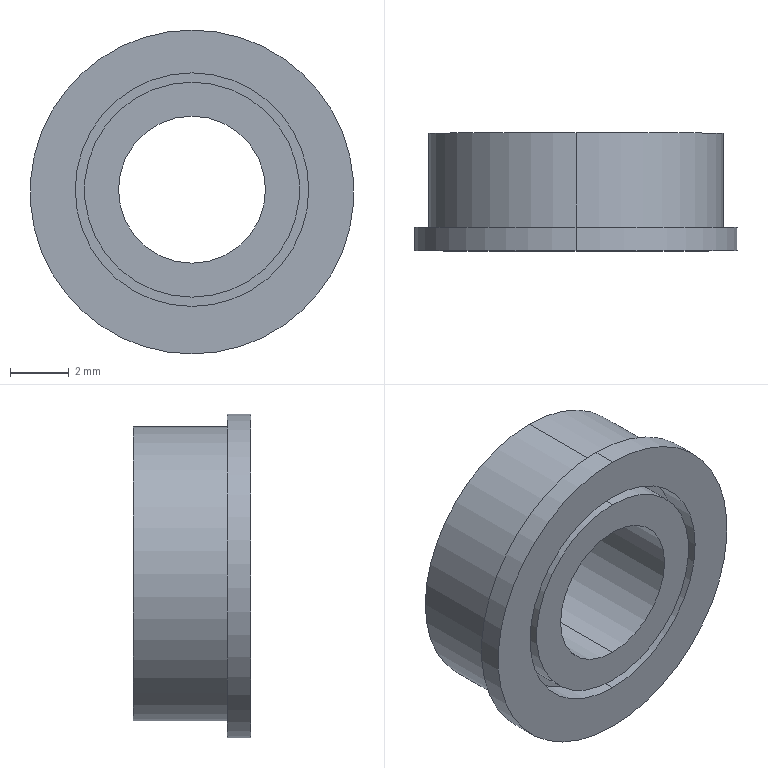Part | STEP file | Flange bearing 5104 | 1 solid | 21 faces | box 11 x 4 x 11 mm | volume 233.729 mm3 | cylinder 14 | plane 7 | commonest cylinder face diameters 7.305 x4 7.935 x4 5 x2 10 x2 11 x2
STEP:
#1=CARTESIAN_POINT('',(0.,0.,0.));
#2=DIRECTION('',(0.,0.,1.));
#3=DIRECTION('',(1.,0.,0.));
#4=AXIS2_PLACEMENT_3D('',#1,#2,#3);
#5=CARTESIAN_POINT('',(0.,1.,-3.653));
#6=VERTEX_POINT('',#5);
#7=CARTESIAN_POINT('',(0.,1.,3.653));
#8=VERTEX_POINT('',#7);
#9=CARTESIAN_POINT('',(0.,1.,0.));
#10=DIRECTION('',(0.,-1.,0.));
#11=DIRECTION('',(0.,0.,-1.));
#12=AXIS2_PLACEMENT_3D('',#9,#10,#11);
#13=CIRCLE('',#12,3.653);
#14=CARTESIAN_POINT('',(0.,1.,0.));
#15=DIRECTION('',(0.,-1.,0.));
#16=DIRECTION('',(0.,0.,-1.));
#17=AXIS2_PLACEMENT_3D('',#14,#15,#16);
#18=CYLINDRICAL_SURFACE('',#17,3.653);
#19=CARTESIAN_POINT('',(0.,0.));
#20=DIRECTION('',(1.,0.));
#21=VECTOR('',#20,1.);
#22=LINE('',#19,#21);
#23=(GEOMETRIC_REPRESENTATION_CONTEXT(2)PARAMETRIC_REPRESENTATION_CONTEXT()REPRESENTATION_CONTEXT('',''));
#24=DEFINITIONAL_REPRESENTATION('',(#22),#23);
#25=PCURVE('',#18,#24);
#26=CARTESIAN_POINT('',(0.,1.,0.));
#27=DIRECTION('',(0.,-1.,0.));
#28=DIRECTION('',(0.,0.,-1.));
#29=AXIS2_PLACEMENT_3D('',#26,#27,#28);
#30=PLANE('',#29);
#31=CARTESIAN_POINT('',(0.,0.));
#32=DIRECTION('',(1.,0.));
#33=AXIS2_PLACEMENT_2D('',#31,#32);
#34=CIRCLE('',#33,3.653);
#35=(GEOMETRIC_REPRESENTATION_CONTEXT(2)PARAMETRIC_REPRESENTATION_CONTEXT()REPRESENTATION_CONTEXT('',''));
#36=DEFINITIONAL_REPRESENTATION('',(#34),#35);
#37=PCURVE('',#30,#36);
#38=SURFACE_CURVE('',#13,(#25,#37),.PCURVE_S1.);
#39=EDGE_CURVE('',#6,#8,#38,.T.);
#40=ORIENTED_EDGE('',*,*,#39,.T.);
#41=CARTESIAN_POINT('',(0.,0.,3.653));
#42=VERTEX_POINT('',#41);
#43=CARTESIAN_POINT('',(0.,1.,3.653));
#44=DIRECTION('',(0.,-1.,0.));
#45=VECTOR('',#44,1.);
#46=LINE('',#43,#45);
#47=CARTESIAN_POINT('',(3.142,0.));
#48=DIRECTION('',(0.,1.));
#49=VECTOR('',#48,1.);
#50=LINE('',#47,#49);
#51=(GEOMETRIC_REPRESENTATION_CONTEXT(2)PARAMETRIC_REPRESENTATION_CONTEXT()REPRESENTATION_CONTEXT('',''));
#52=DEFINITIONAL_REPRESENTATION('',(#50),#51);
#53=PCURVE('',#18,#52);
#54=CARTESIAN_POINT('',(0.,1.,0.));
#55=DIRECTION('',(0.,-1.,0.));
#56=DIRECTION('',(0.,0.,-1.));
#57=AXIS2_PLACEMENT_3D('',#54,#55,#56);
#58=CYLINDRICAL_SURFACE('',#57,3.653);
#59=CARTESIAN_POINT('',(3.142,0.));
#60=DIRECTION('',(0.,1.));
#61=VECTOR('',#60,1.);
#62=LINE('',#59,#61);
#63=(GEOMETRIC_REPRESENTATION_CONTEXT(2)PARAMETRIC_REPRESENTATION_CONTEXT()REPRESENTATION_CONTEXT('',''));
#64=DEFINITIONAL_REPRESENTATION('',(#62),#63);
#65=PCURVE('',#58,#64);
#66=SURFACE_CURVE('',#46,(#53,#65),.PCURVE_S1.);
#67=EDGE_CURVE('',#8,#42,#66,.T.);
#68=ORIENTED_EDGE('',*,*,#67,.T.);
#69=CARTESIAN_POINT('',(0.,0.,-3.653));
#70=VERTEX_POINT('',#69);
#71=CARTESIAN_POINT('',(0.,0.,0.));
#72=DIRECTION('',(0.,-1.,0.));
#73=DIRECTION('',(0.,0.,-1.));
#74=AXIS2_PLACEMENT_3D('',#71,#72,#73);
#75=CIRCLE('',#74,3.653);
#76=CARTESIAN_POINT('',(0.,1.));
#77=DIRECTION('',(1.,0.));
#78=VECTOR('',#77,1.);
#79=LINE('',#76,#78);
#80=(GEOMETRIC_REPRESENTATION_CONTEXT(2)PARAMETRIC_REPRESENTATION_CONTEXT()REPRESENTATION_CONTEXT('',''));
#81=DEFINITIONAL_REPRESENTATION('',(#79),#80);
#82=PCURVE('',#18,#81);
#83=CARTESIAN_POINT('',(0.,0.,0.));
#84=DIRECTION('',(0.,1.,0.));
#85=DIRECTION('',(0.,0.,1.));
#86=AXIS2_PLACEMENT_3D('',#83,#84,#85);
#87=PLANE('',#86);
#88=CARTESIAN_POINT('',(-3.653,0.));
#89=CARTESIAN_POINT('',(-3.653,6.326));
#90=CARTESIAN_POINT('',(1.826,3.163));
#91=CARTESIAN_POINT('',(7.305,0.));
#92=CARTESIAN_POINT('',(1.826,-3.163));
#93=CARTESIAN_POINT('',(-3.653,-6.326));
#94=CARTESIAN_POINT('',(-3.653,0.));
#95=(BOUNDED_CURVE()B_SPLINE_CURVE(2,(#88,#89,#90,#91,#92,#93,#94),.UNSPECIFIED.,.T.,.F.)B_SPLINE_CURVE_WITH_KNOTS((1,2,2,2,2,1),(-2.094,0.,2.094,4.189,6.283,8.378),.UNSPECIFIED.)CURVE()GEOMETRIC_REPRESENTATION_ITEM()RATIONAL_B_SPLINE_CURVE((1.,0.5,1.,0.5,1.,0.5,1.))REPRESENTATION_ITEM(''));
#96=(GEOMETRIC_REPRESENTATION_CONTEXT(2)PARAMETRIC_REPRESENTATION_CONTEXT()REPRESENTATION_CONTEXT('',''));
#97=DEFINITIONAL_REPRESENTATION('',(#95),#96);
#98=PCURVE('',#87,#97);
#99=SURFACE_CURVE('',#75,(#82,#98),.PCURVE_S1.);
#100=EDGE_CURVE('',#70,#42,#99,.T.);
#101=ORIENTED_EDGE('',*,*,#100,.F.);
#102=CARTESIAN_POINT('',(0.,1.,-3.653));
#103=DIRECTION('',(0.,-1.,0.));
#104=VECTOR('',#103,1.);
#105=LINE('',#102,#104);
#106=CARTESIAN_POINT('',(0.,0.));
#107=DIRECTION('',(0.,1.));
#108=VECTOR('',#107,1.);
#109=LINE('',#106,#108);
#110=(GEOMETRIC_REPRESENTATION_CONTEXT(2)PARAMETRIC_REPRESENTATION_CONTEXT()REPRESENTATION_CONTEXT('',''));
#111=DEFINITIONAL_REPRESENTATION('',(#109),#110);
#112=PCURVE('',#18,#111);
#113=CARTESIAN_POINT('',(6.283,0.));
#114=DIRECTION('',(0.,1.));
#115=VECTOR('',#114,1.);
#116=LINE('',#113,#115);
#117=(GEOMETRIC_REPRESENTATION_CONTEXT(2)PARAMETRIC_REPRESENTATION_CONTEXT()REPRESENTATION_CONTEXT('',''));
#118=DEFINITIONAL_REPRESENTATION('',(#116),#117);
#119=PCURVE('',#58,#118);
#120=SURFACE_CURVE('',#105,(#112,#119),.PCURVE_S1.);
#121=EDGE_CURVE('',#6,#70,#120,.T.);
#122=ORIENTED_EDGE('',*,*,#121,.F.);
#123=EDGE_LOOP('',(#40,#68,#101,#122));
#124=FACE_BOUND('',#123,.T.);
#125=ADVANCED_FACE('',(#124),#18,.T.);
#126=CARTESIAN_POINT('',(0.,1.,-3.968));
#127=VERTEX_POINT('',#126);
#128=CARTESIAN_POINT('',(0.,0.,-3.968));
#129=VERTEX_POINT('',#128);
#130=CARTESIAN_POINT('',(0.,1.,-3.968));
#131=DIRECTION('',(0.,-1.,0.));
#132=VECTOR('',#131,1.);
#133=LINE('',#130,#132);
#134=CARTESIAN_POINT('',(0.,1.,0.));
#135=DIRECTION('',(0.,-1.,0.));
#136=DIRECTION('',(0.,0.,-1.));
#137=AXIS2_PLACEMENT_3D('',#134,#135,#136);
#138=CYLINDRICAL_SURFACE('',#137,3.968);
#139=CARTESIAN_POINT('',(6.283,0.));
#140=DIRECTION('',(0.,1.));
#141=VECTOR('',#140,1.);
#142=LINE('',#139,#141);
#143=(GEOMETRIC_REPRESENTATION_CONTEXT(2)PARAMETRIC_REPRESENTATION_CONTEXT()REPRESENTATION_CONTEXT('',''));
#144=DEFINITIONAL_REPRESENTATION('',(#142),#143);
#145=PCURVE('',#138,#144);
#146=CARTESIAN_POINT('',(0.,1.,0.));
#147=DIRECTION('',(0.,-1.,0.));
#148=DIRECTION('',(0.,0.,-1.));
#149=AXIS2_PLACEMENT_3D('',#146,#147,#148);
#150=CYLINDRICAL_SURFACE('',#149,3.968);
#151=CARTESIAN_POINT('',(0.,0.));
#152=DIRECTION('',(0.,1.));
#153=VECTOR('',#152,1.);
#154=LINE('',#151,#153);
#155=(GEOMETRIC_REPRESENTATION_CONTEXT(2)PARAMETRIC_REPRESENTATION_CONTEXT()REPRESENTATION_CONTEXT('',''));
#156=DEFINITIONAL_REPRESENTATION('',(#154),#155);
#157=PCURVE('',#150,#156);
#158=SURFACE_CURVE('',#133,(#145,#157),.PCURVE_S1.);
#159=EDGE_CURVE('',#127,#129,#158,.T.);
#160=ORIENTED_EDGE('',*,*,#159,.T.);
#161=CARTESIAN_POINT('',(0.,0.,3.968));
#162=VERTEX_POINT('',#161);
#163=CARTESIAN_POINT('',(0.,0.,0.));
#164=DIRECTION('',(0.,-1.,0.));
#165=DIRECTION('',(0.,0.,-1.));
#166=AXIS2_PLACEMENT_3D('',#163,#164,#165);
#167=CIRCLE('',#166,3.968);
#168=CARTESIAN_POINT('',(0.,1.));
#169=DIRECTION('',(1.,0.));
#170=VECTOR('',#169,1.);
#171=LINE('',#168,#170);
#172=(GEOMETRIC_REPRESENTATION_CONTEXT(2)PARAMETRIC_REPRESENTATION_CONTEXT()REPRESENTATION_CONTEXT('',''));
#173=DEFINITIONAL_REPRESENTATION('',(#171),#172);
#174=PCURVE('',#138,#173);
#175=CARTESIAN_POINT('',(0.,0.,0.));
#176=DIRECTION('',(0.,1.,0.));
#177=DIRECTION('',(0.,0.,1.));
#178=AXIS2_PLACEMENT_3D('',#175,#176,#177);
#179=PLANE('',#178);
#180=CARTESIAN_POINT('',(-3.968,0.));
#181=CARTESIAN_POINT('',(-3.968,6.872));
#182=CARTESIAN_POINT('',(1.984,3.436));
#183=CARTESIAN_POINT('',(7.935,0.));
#184=CARTESIAN_POINT('',(1.984,-3.436));
#185=CARTESIAN_POINT('',(-3.968,-6.872));
#186=CARTESIAN_POINT('',(-3.968,0.));
#187=(BOUNDED_CURVE()B_SPLINE_CURVE(2,(#180,#181,#182,#183,#184,#185,#186),.UNSPECIFIED.,.T.,.F.)B_SPLINE_CURVE_WITH_KNOTS((1,2,2,2,2,1),(-2.094,0.,2.094,4.189,6.283,8.378),.UNSPECIFIED.)CURVE()GEOMETRIC_REPRESENTATION_ITEM()RATIONAL_B_SPLINE_CURVE((1.,0.5,1.,0.5,1.,0.5,1.))REPRESENTATION_ITEM(''));
#188=(GEOMETRIC_REPRESENTATION_CONTEXT(2)PARAMETRIC_REPRESENTATION_CONTEXT()REPRESENTATION_CONTEXT('',''));
#189=DEFINITIONAL_REPRESENTATION('',(#187),#188);
#190=PCURVE('',#179,#189);
#191=SURFACE_CURVE('',#167,(#174,#190),.PCURVE_S1.);
#192=EDGE_CURVE('',#162,#129,#191,.T.);
#193=ORIENTED_EDGE('',*,*,#192,.F.);
#194=CARTESIAN_POINT('',(0.,1.,3.968));
#195=VERTEX_POINT('',#194);
#196=CARTESIAN_POINT('',(0.,1.,3.968));
#197=DIRECTION('',(0.,-1.,0.));
#198=VECTOR('',#197,1.);
#199=LINE('',#196,#198);
#200=CARTESIAN_POINT('',(3.142,0.));
#201=DIRECTION('',(0.,1.));
#202=VECTOR('',#201,1.);
#203=LINE('',#200,#202);
#204=(GEOMETRIC_REPRESENTATION_CONTEXT(2)PARAMETRIC_REPRESENTATION_CONTEXT()REPRESENTATION_CONTEXT('',''));
#205=DEFINITIONAL_REPRESENTATION('',(#203),#204);
#206=PCURVE('',#138,#205);
#207=CARTESIAN_POINT('',(3.142,0.));
#208=DIRECTION('',(0.,1.));
#209=VECTOR('',#208,1.);
#210=LINE('',#207,#209);
#211=(GEOMETRIC_REPRESENTATION_CONTEXT(2)PARAMETRIC_REPRESENTATION_CONTEXT()REPRESENTATION_CONTEXT('',''));
#212=DEFINITIONAL_REPRESENTATION('',(#210),#211);
#213=PCURVE('',#150,#212);
#214=SURFACE_CURVE('',#199,(#206,#213),.PCURVE_S1.);
#215=EDGE_CURVE('',#195,#162,#214,.T.);
#216=ORIENTED_EDGE('',*,*,#215,.F.);
#217=CARTESIAN_POINT('',(0.,1.,0.));
#218=DIRECTION('',(0.,-1.,0.));
#219=DIRECTION('',(0.,0.,-1.));
#220=AXIS2_PLACEMENT_3D('',#217,#218,#219);
#221=CIRCLE('',#220,3.968);
#222=CARTESIAN_POINT('',(0.,0.));
#223=DIRECTION('',(1.,0.));
#224=VECTOR('',#223,1.);
#225=LINE('',#222,#224);
#226=(GEOMETRIC_REPRESENTATION_CONTEXT(2)PARAMETRIC_REPRESENTATION_CONTEXT()REPRESENTATION_CONTEXT('',''));
#227=DEFINITIONAL_REPRESENTATION('',(#225),#226);
#228=PCURVE('',#138,#227);
#229=CARTESIAN_POINT('',(0.,0.));
#230=DIRECTION('',(1.,0.));
#231=AXIS2_PLACEMENT_2D('',#229,#230);
#232=CIRCLE('',#231,3.968);
#233=(GEOMETRIC_REPRESENTATION_CONTEXT(2)PARAMETRIC_REPRESENTATION_CONTEXT()REPRESENTATION_CONTEXT('',''));
#234=DEFINITIONAL_REPRESENTATION('',(#232),#233);
#235=PCURVE('',#30,#234);
#236=SURFACE_CURVE('',#221,(#228,#235),.PCURVE_S1.);
#237=EDGE_CURVE('',#195,#127,#236,.T.);
#238=ORIENTED_EDGE('',*,*,#237,.T.);
#239=EDGE_LOOP('',(#160,#193,#216,#238));
#240=FACE_BOUND('',#239,.F.);
#241=ADVANCED_FACE('',(#240),#138,.F.);
#242=CARTESIAN_POINT('',(0.,0.8,-5.58));
#243=VERTEX_POINT('',#242);
#244=CARTESIAN_POINT('',(0.,0.8,5.42));
#245=VERTEX_POINT('',#244);
#246=CARTESIAN_POINT('',(0.,0.8,-0.07954));
#247=DIRECTION('',(0.,-1.,0.));
#248=DIRECTION('',(0.,0.,-1.));
#249=AXIS2_PLACEMENT_3D('',#246,#247,#248);
#250=CIRCLE('',#249,5.5);
#251=CARTESIAN_POINT('',(0.,0.8,-0.07954));
#252=DIRECTION('',(0.,-1.,0.));
#253=DIRECTION('',(0.,0.,-1.));
#254=AXIS2_PLACEMENT_3D('',#251,#252,#253);
#255=CYLINDRICAL_SURFACE('',#254,5.5);
#256=CARTESIAN_POINT('',(0.,0.));
#257=DIRECTION('',(1.,0.));
#258=VECTOR('',#257,1.);
#259=LINE('',#256,#258);
#260=(GEOMETRIC_REPRESENTATION_CONTEXT(2)PARAMETRIC_REPRESENTATION_CONTEXT()REPRESENTATION_CONTEXT('',''));
#261=DEFINITIONAL_REPRESENTATION('',(#259),#260);
#262=PCURVE('',#255,#261);
#263=CARTESIAN_POINT('',(0.,0.8,-0.07954));
#264=DIRECTION('',(0.,-1.,0.));
#265=DIRECTION('',(0.,0.,-1.));
#266=AXIS2_PLACEMENT_3D('',#263,#264,#265);
#267=PLANE('',#266);
#268=CARTESIAN_POINT('',(0.,0.));
#269=DIRECTION('',(1.,0.));
#270=AXIS2_PLACEMENT_2D('',#268,#269);
#271=CIRCLE('',#270,5.5);
#272=(GEOMETRIC_REPRESENTATION_CONTEXT(2)PARAMETRIC_REPRESENTATION_CONTEXT()REPRESENTATION_CONTEXT('',''));
#273=DEFINITIONAL_REPRESENTATION('',(#271),#272);
#274=PCURVE('',#267,#273);
#275=SURFACE_CURVE('',#250,(#262,#274),.PCURVE_S1.);
#276=EDGE_CURVE('',#243,#245,#275,.T.);
#277=ORIENTED_EDGE('',*,*,#276,.T.);
#278=CARTESIAN_POINT('',(0.,0.,5.42));
#279=VERTEX_POINT('',#278);
#280=CARTESIAN_POINT('',(0.,0.8,5.42));
#281=DIRECTION('',(0.,-1.,0.));
#282=VECTOR('',#281,1.);
#283=LINE('',#280,#282);
#284=CARTESIAN_POINT('',(3.142,0.));
#285=DIRECTION('',(0.,1.));
#286=VECTOR('',#285,1.);
#287=LINE('',#284,#286);
#288=(GEOMETRIC_REPRESENTATION_CONTEXT(2)PARAMETRIC_REPRESENTATION_CONTEXT()REPRESENTATION_CONTEXT('',''));
#289=DEFINITIONAL_REPRESENTATION('',(#287),#288);
#290=PCURVE('',#255,#289);
#291=CARTESIAN_POINT('',(0.,0.8,-0.07954));
#292=DIRECTION('',(0.,-1.,0.));
#293=DIRECTION('',(0.,0.,-1.));
#294=AXIS2_PLACEMENT_3D('',#291,#292,#293);
#295=CYLINDRICAL_SURFACE('',#294,5.5);
#296=CARTESIAN_POINT('',(3.142,0.));
#297=DIRECTION('',(0.,1.));
#298=VECTOR('',#297,1.);
#299=LINE('',#296,#298);
#300=(GEOMETRIC_REPRESENTATION_CONTEXT(2)PARAMETRIC_REPRESENTATION_CONTEXT()REPRESENTATION_CONTEXT('',''));
#301=DEFINITIONAL_REPRESENTATION('',(#299),#300);
#302=PCURVE('',#295,#301);
#303=SURFACE_CURVE('',#283,(#290,#302),.PCURVE_S1.);
#304=EDGE_CURVE('',#245,#279,#303,.T.);
#305=ORIENTED_EDGE('',*,*,#304,.T.);
#306=CARTESIAN_POINT('',(0.,0.,-5.58));
#307=VERTEX_POINT('',#306);
#308=CARTESIAN_POINT('',(0.,0.,-0.07954));
#309=DIRECTION('',(0.,-1.,0.));
#310=DIRECTION('',(0.,0.,-1.));
#311=AXIS2_PLACEMENT_3D('',#308,#309,#310);
#312=CIRCLE('',#311,5.5);
#313=CARTESIAN_POINT('',(0.,0.8));
#314=DIRECTION('',(1.,0.));
#315=VECTOR('',#314,1.);
#316=LINE('',#313,#315);
#317=(GEOMETRIC_REPRESENTATION_CONTEXT(2)PARAMETRIC_REPRESENTATION_CONTEXT()REPRESENTATION_CONTEXT('',''));
#318=DEFINITIONAL_REPRESENTATION('',(#316),#317);
#319=PCURVE('',#255,#318);
#320=CARTESIAN_POINT('',(-5.58,0.));
#321=CARTESIAN_POINT('',(-5.58,9.526));
#322=CARTESIAN_POINT('',(2.67,4.763));
#323=CARTESIAN_POINT('',(10.92,0.));
#324=CARTESIAN_POINT('',(2.67,-4.763));
#325=CARTESIAN_POINT('',(-5.58,-9.526));
#326=CARTESIAN_POINT('',(-5.58,0.));
#327=(BOUNDED_CURVE()B_SPLINE_CURVE(2,(#320,#321,#322,#323,#324,#325,#326),.UNSPECIFIED.,.T.,.F.)B_SPLINE_CURVE_WITH_KNOTS((1,2,2,2,2,1),(-2.094,0.,2.094,4.189,6.283,8.378),.UNSPECIFIED.)CURVE()GEOMETRIC_REPRESENTATION_ITEM()RATIONAL_B_SPLINE_CURVE((1.,0.5,1.,0.5,1.,0.5,1.))REPRESENTATION_ITEM(''));
#328=(GEOMETRIC_REPRESENTATION_CONTEXT(2)PARAMETRIC_REPRESENTATION_CONTEXT()REPRESENTATION_CONTEXT('',''));
#329=DEFINITIONAL_REPRESENTATION('',(#327),#328);
#330=PCURVE('',#179,#329);
#331=SURFACE_CURVE('',#312,(#319,#330),.PCURVE_S1.);
#332=EDGE_CURVE('',#307,#279,#331,.T.);
#333=ORIENTED_EDGE('',*,*,#332,.F.);
#334=CARTESIAN_POINT('',(0.,0.8,-5.58));
#335=DIRECTION('',(0.,-1.,0.));
#336=VECTOR('',#335,1.);
#337=LINE('',#334,#336);
#338=CARTESIAN_POINT('',(0.,0.));
#339=DIRECTION('',(0.,1.));
#340=VECTOR('',#339,1.);
#341=LINE('',#338,#340);
#342=(GEOMETRIC_REPRESENTATION_CONTEXT(2)PARAMETRIC_REPRESENTATION_CONTEXT()REPRESENTATION_CONTEXT('',''));
#343=DEFINITIONAL_REPRESENTATION('',(#341),#342);
#344=PCURVE('',#255,#343);
#345=CARTESIAN_POINT('',(6.283,0.));
#346=DIRECTION('',(0.,1.));
#347=VECTOR('',#346,1.);
#348=LINE('',#345,#347);
#349=(GEOMETRIC_REPRESENTATION_CONTEXT(2)PARAMETRIC_REPRESENTATION_CONTEXT()REPRESENTATION_CONTEXT('',''));
#350=DEFINITIONAL_REPRESENTATION('',(#348),#349);
#351=PCURVE('',#295,#350);
#352=SURFACE_CURVE('',#337,(#344,#351),.PCURVE_S1.);
#353=EDGE_CURVE('',#243,#307,#352,.T.);
#354=ORIENTED_EDGE('',*,*,#353,.F.);
#355=EDGE_LOOP('',(#277,#305,#333,#354));
#356=FACE_BOUND('',#355,.T.);
#357=ADVANCED_FACE('',(#356),#255,.T.);
#358=CARTESIAN_POINT('',(0.,4.,-2.5));
#359=VERTEX_POINT('',#358);
#360=CARTESIAN_POINT('',(0.,0.,-2.5));
#361=VERTEX_POINT('',#360);
#362=CARTESIAN_POINT('',(0.,4.,-2.5));
#363=DIRECTION('',(0.,-1.,0.));
#364=VECTOR('',#363,1.);
#365=LINE('',#362,#364);
#366=CARTESIAN_POINT('',(0.,4.,0.));
#367=DIRECTION('',(0.,-1.,0.));
#368=DIRECTION('',(0.,0.,-1.));
#369=AXIS2_PLACEMENT_3D('',#366,#367,#368);
#370=CYLINDRICAL_SURFACE('',#369,2.5);
#371=CARTESIAN_POINT('',(6.283,0.));
#372=DIRECTION('',(0.,1.));
#373=VECTOR('',#372,1.);
#374=LINE('',#371,#373);
#375=(GEOMETRIC_REPRESENTATION_CONTEXT(2)PARAMETRIC_REPRESENTATION_CONTEXT()REPRESENTATION_CONTEXT('',''));
#376=DEFINITIONAL_REPRESENTATION('',(#374),#375);
#377=PCURVE('',#370,#376);
#378=CARTESIAN_POINT('',(0.,4.,0.));
#379=DIRECTION('',(0.,-1.,0.));
#380=DIRECTION('',(0.,0.,-1.));
#381=AXIS2_PLACEMENT_3D('',#378,#379,#380);
#382=CYLINDRICAL_SURFACE('',#381,2.5);
#383=CARTESIAN_POINT('',(0.,0.));
#384=DIRECTION('',(0.,1.));
#385=VECTOR('',#384,1.);
#386=LINE('',#383,#385);
#387=(GEOMETRIC_REPRESENTATION_CONTEXT(2)PARAMETRIC_REPRESENTATION_CONTEXT()REPRESENTATION_CONTEXT('',''));
#388=DEFINITIONAL_REPRESENTATION('',(#386),#387);
#389=PCURVE('',#382,#388);
#390=SURFACE_CURVE('',#365,(#377,#389),.PCURVE_S1.);
#391=EDGE_CURVE('',#359,#361,#390,.T.);
#392=ORIENTED_EDGE('',*,*,#391,.T.);
#393=CARTESIAN_POINT('',(0.,0.,2.5));
#394=VERTEX_POINT('',#393);
#395=CARTESIAN_POINT('',(0.,0.,0.));
#396=DIRECTION('',(0.,1.,0.));
#397=DIRECTION('',(0.,0.,1.));
#398=AXIS2_PLACEMENT_3D('',#395,#396,#397);
#399=CIRCLE('',#398,2.5);
#400=CARTESIAN_POINT('',(9.425,4.));
#401=DIRECTION('',(-1.,0.));
#402=VECTOR('',#401,1.);
#403=LINE('',#400,#402);
#404=(GEOMETRIC_REPRESENTATION_CONTEXT(2)PARAMETRIC_REPRESENTATION_CONTEXT()REPRESENTATION_CONTEXT('',''));
#405=DEFINITIONAL_REPRESENTATION('',(#403),#404);
#406=PCURVE('',#370,#405);
#407=CARTESIAN_POINT('',(0.,0.));
#408=DIRECTION('',(1.,0.));
#409=AXIS2_PLACEMENT_2D('',#407,#408);
#410=CIRCLE('',#409,2.5);
#411=(GEOMETRIC_REPRESENTATION_CONTEXT(2)PARAMETRIC_REPRESENTATION_CONTEXT()REPRESENTATION_CONTEXT('',''));
#412=DEFINITIONAL_REPRESENTATION('',(#410),#411);
#413=PCURVE('',#87,#412);
#414=SURFACE_CURVE('',#399,(#406,#413),.PCURVE_S1.);
#415=EDGE_CURVE('',#361,#394,#414,.T.);
#416=ORIENTED_EDGE('',*,*,#415,.T.);
#417=CARTESIAN_POINT('',(0.,4.,2.5));
#418=VERTEX_POINT('',#417);
#419=CARTESIAN_POINT('',(0.,4.,2.5));
#420=DIRECTION('',(0.,-1.,0.));
#421=VECTOR('',#420,1.);
#422=LINE('',#419,#421);
#423=CARTESIAN_POINT('',(3.142,0.));
#424=DIRECTION('',(0.,1.));
#425=VECTOR('',#424,1.);
#426=LINE('',#423,#425);
#427=(GEOMETRIC_REPRESENTATION_CONTEXT(2)PARAMETRIC_REPRESENTATION_CONTEXT()REPRESENTATION_CONTEXT('',''));
#428=DEFINITIONAL_REPRESENTATION('',(#426),#427);
#429=PCURVE('',#370,#428);
#430=CARTESIAN_POINT('',(3.142,0.));
#431=DIRECTION('',(0.,1.));
#432=VECTOR('',#431,1.);
#433=LINE('',#430,#432);
#434=(GEOMETRIC_REPRESENTATION_CONTEXT(2)PARAMETRIC_REPRESENTATION_CONTEXT()REPRESENTATION_CONTEXT('',''));
#435=DEFINITIONAL_REPRESENTATION('',(#433),#434);
#436=PCURVE('',#382,#435);
#437=SURFACE_CURVE('',#422,(#429,#436),.PCURVE_S1.);
#438=EDGE_CURVE('',#418,#394,#437,.T.);
#439=ORIENTED_EDGE('',*,*,#438,.F.);
#440=CARTESIAN_POINT('',(0.,4.,0.));
#441=DIRECTION('',(0.,1.,0.));
#442=DIRECTION('',(0.,0.,1.));
#443=AXIS2_PLACEMENT_3D('',#440,#441,#442);
#444=CIRCLE('',#443,2.5);
#445=CARTESIAN_POINT('',(9.425,0.));
#446=DIRECTION('',(-1.,0.));
#447=VECTOR('',#446,1.);
#448=LINE('',#445,#447);
#449=(GEOMETRIC_REPRESENTATION_CONTEXT(2)PARAMETRIC_REPRESENTATION_CONTEXT()REPRESENTATION_CONTEXT('',''));
#450=DEFINITIONAL_REPRESENTATION('',(#448),#449);
#451=PCURVE('',#370,#450);
#452=CARTESIAN_POINT('',(0.,4.,0.));
#453=DIRECTION('',(0.,1.,0.));
#454=DIRECTION('',(0.,0.,1.));
#455=AXIS2_PLACEMENT_3D('',#452,#453,#454);
#456=PLANE('',#455);
#457=CARTESIAN_POINT('',(0.,0.));
#458=DIRECTION('',(1.,0.));
#459=AXIS2_PLACEMENT_2D('',#457,#458);
#460=CIRCLE('',#459,2.5);
#461=(GEOMETRIC_REPRESENTATION_CONTEXT(2)PARAMETRIC_REPRESENTATION_CONTEXT()REPRESENTATION_CONTEXT('',''));
#462=DEFINITIONAL_REPRESENTATION('',(#460),#461);
#463=PCURVE('',#456,#462);
#464=SURFACE_CURVE('',#444,(#451,#463),.PCURVE_S1.);
#465=EDGE_CURVE('',#359,#418,#464,.T.);
#466=ORIENTED_EDGE('',*,*,#465,.F.);
#467=EDGE_LOOP('',(#392,#416,#439,#466));
#468=FACE_BOUND('',#467,.F.);
#469=ADVANCED_FACE('',(#468),#370,.F.);
#470=CARTESIAN_POINT('',(0.,4.,5.));
#471=VERTEX_POINT('',#470);
#472=CARTESIAN_POINT('',(0.,4.,-5.));
#473=VERTEX_POINT('',#472);
#474=CARTESIAN_POINT('',(0.,4.,0.));
#475=DIRECTION('',(0.,1.,0.));
#476=DIRECTION('',(0.,0.,1.));
#477=AXIS2_PLACEMENT_3D('',#474,#475,#476);
#478=CIRCLE('',#477,5.);
#479=CARTESIAN_POINT('',(0.,4.,0.));
#480=DIRECTION('',(0.,-1.,0.));
#481=DIRECTION('',(0.,0.,-1.));
#482=AXIS2_PLACEMENT_3D('',#479,#480,#481);
#483=CYLINDRICAL_SURFACE('',#482,5.);
#484=CARTESIAN_POINT('',(3.142,0.));
#485=DIRECTION('',(-1.,0.));
#486=VECTOR('',#485,1.);
#487=LINE('',#484,#486);
#488=(GEOMETRIC_REPRESENTATION_CONTEXT(2)PARAMETRIC_REPRESENTATION_CONTEXT()REPRESENTATION_CONTEXT('',''));
#489=DEFINITIONAL_REPRESENTATION('',(#487),#488);
#490=PCURVE('',#483,#489);
#491=CARTESIAN_POINT('',(0.,0.));
#492=DIRECTION('',(1.,0.));
#493=AXIS2_PLACEMENT_2D('',#491,#492);
#494=CIRCLE('',#493,5.);
#495=(GEOMETRIC_REPRESENTATION_CONTEXT(2)PARAMETRIC_REPRESENTATION_CONTEXT()REPRESENTATION_CONTEXT('',''));
#496=DEFINITIONAL_REPRESENTATION('',(#494),#495);
#497=PCURVE('',#456,#496);
#498=SURFACE_CURVE('',#478,(#490,#497),.PCURVE_S1.);
#499=EDGE_CURVE('',#471,#473,#498,.T.);
#500=ORIENTED_EDGE('',*,*,#499,.F.);
#501=CARTESIAN_POINT('',(0.,0.8,5.));
#502=VERTEX_POINT('',#501);
#503=CARTESIAN_POINT('',(0.,4.,5.));
#504=DIRECTION('',(0.,-1.,0.));
#505=VECTOR('',#504,1.);
#506=LINE('',#503,#505);
#507=CARTESIAN_POINT('',(3.142,0.));
#508=DIRECTION('',(0.,1.));
#509=VECTOR('',#508,1.);
#510=LINE('',#507,#509);
#511=(GEOMETRIC_REPRESENTATION_CONTEXT(2)PARAMETRIC_REPRESENTATION_CONTEXT()REPRESENTATION_CONTEXT('',''));
#512=DEFINITIONAL_REPRESENTATION('',(#510),#511);
#513=PCURVE('',#483,#512);
#514=CARTESIAN_POINT('',(0.,4.,0.));
#515=DIRECTION('',(0.,-1.,0.));
#516=DIRECTION('',(0.,0.,-1.));
#517=AXIS2_PLACEMENT_3D('',#514,#515,#516);
#518=CYLINDRICAL_SURFACE('',#517,5.);
#519=CARTESIAN_POINT('',(3.142,0.));
#520=DIRECTION('',(0.,1.));
#521=VECTOR('',#520,1.);
#522=LINE('',#519,#521);
#523=(GEOMETRIC_REPRESENTATION_CONTEXT(2)PARAMETRIC_REPRESENTATION_CONTEXT()REPRESENTATION_CONTEXT('',''));
#524=DEFINITIONAL_REPRESENTATION('',(#522),#523);
#525=PCURVE('',#518,#524);
#526=SURFACE_CURVE('',#506,(#513,#525),.PCURVE_S1.);
#527=EDGE_CURVE('',#471,#502,#526,.T.);
#528=ORIENTED_EDGE('',*,*,#527,.T.);
#529=CARTESIAN_POINT('',(0.,0.8,-5.));
#530=VERTEX_POINT('',#529);
#531=CARTESIAN_POINT('',(0.,0.8,0.));
#532=DIRECTION('',(0.,-1.,0.));
#533=DIRECTION('',(0.,0.,-1.));
#534=AXIS2_PLACEMENT_3D('',#531,#532,#533);
#535=CIRCLE('',#534,5.);
#536=CARTESIAN_POINT('',(0.,3.2));
#537=DIRECTION('',(1.,0.));
#538=VECTOR('',#537,1.);
#539=LINE('',#536,#538);
#540=(GEOMETRIC_REPRESENTATION_CONTEXT(2)PARAMETRIC_REPRESENTATION_CONTEXT()REPRESENTATION_CONTEXT('',''));
#541=DEFINITIONAL_REPRESENTATION('',(#539),#540);
#542=PCURVE('',#483,#541);
#543=CARTESIAN_POINT('',(-0.07954,0.));
#544=DIRECTION('',(1.,0.));
#545=AXIS2_PLACEMENT_2D('',#543,#544);
#546=CIRCLE('',#545,5.);
#547=(GEOMETRIC_REPRESENTATION_CONTEXT(2)PARAMETRIC_REPRESENTATION_CONTEXT()REPRESENTATION_CONTEXT('',''));
#548=DEFINITIONAL_REPRESENTATION('',(#546),#547);
#549=PCURVE('',#267,#548);
#550=SURFACE_CURVE('',#535,(#542,#549),.PCURVE_S1.);
#551=EDGE_CURVE('',#530,#502,#550,.T.);
#552=ORIENTED_EDGE('',*,*,#551,.F.);
#553=CARTESIAN_POINT('',(0.,4.,-5.));
#554=DIRECTION('',(0.,-1.,0.));
#555=VECTOR('',#554,1.);
#556=LINE('',#553,#555);
#557=CARTESIAN_POINT('',(0.,0.));
#558=DIRECTION('',(0.,1.));
#559=VECTOR('',#558,1.);
#560=LINE('',#557,#559);
#561=(GEOMETRIC_REPRESENTATION_CONTEXT(2)PARAMETRIC_REPRESENTATION_CONTEXT()REPRESENTATION_CONTEXT('',''));
#562=DEFINITIONAL_REPRESENTATION('',(#560),#561);
#563=PCURVE('',#483,#562);
#564=CARTESIAN_POINT('',(6.283,0.));
#565=DIRECTION('',(0.,1.));
#566=VECTOR('',#565,1.);
#567=LINE('',#564,#566);
#568=(GEOMETRIC_REPRESENTATION_CONTEXT(2)PARAMETRIC_REPRESENTATION_CONTEXT()REPRESENTATION_CONTEXT('',''));
#569=DEFINITIONAL_REPRESENTATION('',(#567),#568);
#570=PCURVE('',#518,#569);
#571=SURFACE_CURVE('',#556,(#563,#570),.PCURVE_S1.);
#572=EDGE_CURVE('',#473,#530,#571,.T.);
#573=ORIENTED_EDGE('',*,*,#572,.F.);
#574=EDGE_LOOP('',(#500,#528,#552,#573));
#575=FACE_BOUND('',#574,.T.);
#576=ADVANCED_FACE('',(#575),#483,.T.);
#577=ORIENTED_EDGE('',*,*,#415,.T.);
#578=CARTESIAN_POINT('',(0.,0.,0.));
#579=DIRECTION('',(0.,1.,0.));
#580=DIRECTION('',(0.,0.,1.));
#581=AXIS2_PLACEMENT_3D('',#578,#579,#580);
#582=CIRCLE('',#581,2.5);
#583=CARTESIAN_POINT('',(0.,0.));
#584=DIRECTION('',(1.,0.));
#585=AXIS2_PLACEMENT_2D('',#583,#584);
#586=CIRCLE('',#585,2.5);
#587=(GEOMETRIC_REPRESENTATION_CONTEXT(2)PARAMETRIC_REPRESENTATION_CONTEXT()REPRESENTATION_CONTEXT('',''));
#588=DEFINITIONAL_REPRESENTATION('',(#586),#587);
#589=PCURVE('',#87,#588);
#590=CARTESIAN_POINT('',(3.142,4.));
#591=DIRECTION('',(-1.,0.));
#592=VECTOR('',#591,1.);
#593=LINE('',#590,#592);
#594=(GEOMETRIC_REPRESENTATION_CONTEXT(2)PARAMETRIC_REPRESENTATION_CONTEXT()REPRESENTATION_CONTEXT('',''));
#595=DEFINITIONAL_REPRESENTATION('',(#593),#594);
#596=PCURVE('',#382,#595);
#597=SURFACE_CURVE('',#582,(#589,#596),.PCURVE_S1.);
#598=EDGE_CURVE('',#394,#361,#597,.T.);
#599=ORIENTED_EDGE('',*,*,#598,.T.);
#600=EDGE_LOOP('',(#577,#599));
#601=FACE_BOUND('',#600,.T.);
#602=ORIENTED_EDGE('',*,*,#100,.T.);
#603=CARTESIAN_POINT('',(0.,0.,0.));
#604=DIRECTION('',(0.,-1.,0.));
#605=DIRECTION('',(0.,0.,-1.));
#606=AXIS2_PLACEMENT_3D('',#603,#604,#605);
#607=CIRCLE('',#606,3.653);
#608=CARTESIAN_POINT('',(-3.653,0.));
#609=CARTESIAN_POINT('',(-3.653,6.326));
#610=CARTESIAN_POINT('',(1.826,3.163));
#611=CARTESIAN_POINT('',(7.305,0.));
#612=CARTESIAN_POINT('',(1.826,-3.163));
#613=CARTESIAN_POINT('',(-3.653,-6.326));
#614=CARTESIAN_POINT('',(-3.653,0.));
#615=(BOUNDED_CURVE()B_SPLINE_CURVE(2,(#608,#609,#610,#611,#612,#613,#614),.UNSPECIFIED.,.T.,.F.)B_SPLINE_CURVE_WITH_KNOTS((1,2,2,2,2,1),(-2.094,0.,2.094,4.189,6.283,8.378),.UNSPECIFIED.)CURVE()GEOMETRIC_REPRESENTATION_ITEM()RATIONAL_B_SPLINE_CURVE((1.,0.5,1.,0.5,1.,0.5,1.))REPRESENTATION_ITEM(''));
#616=(GEOMETRIC_REPRESENTATION_CONTEXT(2)PARAMETRIC_REPRESENTATION_CONTEXT()REPRESENTATION_CONTEXT('',''));
#617=DEFINITIONAL_REPRESENTATION('',(#615),#616);
#618=PCURVE('',#87,#617);
#619=CARTESIAN_POINT('',(0.,1.));
#620=DIRECTION('',(1.,0.));
#621=VECTOR('',#620,1.);
#622=LINE('',#619,#621);
#623=(GEOMETRIC_REPRESENTATION_CONTEXT(2)PARAMETRIC_REPRESENTATION_CONTEXT()REPRESENTATION_CONTEXT('',''));
#624=DEFINITIONAL_REPRESENTATION('',(#622),#623);
#625=PCURVE('',#58,#624);
#626=SURFACE_CURVE('',#607,(#618,#625),.PCURVE_S1.);
#627=EDGE_CURVE('',#42,#70,#626,.T.);
#628=ORIENTED_EDGE('',*,*,#627,.T.);
#629=EDGE_LOOP('',(#602,#628));
#630=FACE_BOUND('',#629,.T.);
#631=ADVANCED_FACE('',(#601,#630),#87,.F.);
#632=ORIENTED_EDGE('',*,*,#527,.F.);
#633=CARTESIAN_POINT('',(0.,4.,0.));
#634=DIRECTION('',(0.,1.,0.));
#635=DIRECTION('',(0.,0.,1.));
#636=AXIS2_PLACEMENT_3D('',#633,#634,#635);
#637=CIRCLE('',#636,5.);
#638=CARTESIAN_POINT('',(9.425,0.));
#639=DIRECTION('',(-1.,0.));
#640=VECTOR('',#639,1.);
#641=LINE('',#638,#640);
#642=(GEOMETRIC_REPRESENTATION_CONTEXT(2)PARAMETRIC_REPRESENTATION_CONTEXT()REPRESENTATION_CONTEXT('',''));
#643=DEFINITIONAL_REPRESENTATION('',(#641),#642);
#644=PCURVE('',#518,#643);
#645=CARTESIAN_POINT('',(0.,0.));
#646=DIRECTION('',(1.,0.));
#647=AXIS2_PLACEMENT_2D('',#645,#646);
#648=CIRCLE('',#647,5.);
#649=(GEOMETRIC_REPRESENTATION_CONTEXT(2)PARAMETRIC_REPRESENTATION_CONTEXT()REPRESENTATION_CONTEXT('',''));
#650=DEFINITIONAL_REPRESENTATION('',(#648),#649);
#651=PCURVE('',#456,#650);
#652=SURFACE_CURVE('',#637,(#644,#651),.PCURVE_S1.);
#653=EDGE_CURVE('',#473,#471,#652,.T.);
#654=ORIENTED_EDGE('',*,*,#653,.F.);
#655=ORIENTED_EDGE('',*,*,#572,.T.);
#656=CARTESIAN_POINT('',(0.,0.8,0.));
#657=DIRECTION('',(0.,-1.,0.));
#658=DIRECTION('',(0.,0.,-1.));
#659=AXIS2_PLACEMENT_3D('',#656,#657,#658);
#660=CIRCLE('',#659,5.);
#661=CARTESIAN_POINT('',(0.,3.2));
#662=DIRECTION('',(1.,0.));
#663=VECTOR('',#662,1.);
#664=LINE('',#661,#663);
#665=(GEOMETRIC_REPRESENTATION_CONTEXT(2)PARAMETRIC_REPRESENTATION_CONTEXT()REPRESENTATION_CONTEXT('',''));
#666=DEFINITIONAL_REPRESENTATION('',(#664),#665);
#667=PCURVE('',#518,#666);
#668=CARTESIAN_POINT('',(-0.07954,0.));
#669=DIRECTION('',(1.,0.));
#670=AXIS2_PLACEMENT_2D('',#668,#669);
#671=CIRCLE('',#670,5.);
#672=(GEOMETRIC_REPRESENTATION_CONTEXT(2)PARAMETRIC_REPRESENTATION_CONTEXT()REPRESENTATION_CONTEXT('',''));
#673=DEFINITIONAL_REPRESENTATION('',(#671),#672);
#674=PCURVE('',#267,#673);
#675=SURFACE_CURVE('',#660,(#667,#674),.PCURVE_S1.);
#676=EDGE_CURVE('',#502,#530,#675,.T.);
#677=ORIENTED_EDGE('',*,*,#676,.F.);
#678=EDGE_LOOP('',(#632,#654,#655,#677));
#679=FACE_BOUND('',#678,.T.);
#680=ADVANCED_FACE('',(#679),#518,.T.);
#681=ORIENTED_EDGE('',*,*,#653,.T.);
#682=ORIENTED_EDGE('',*,*,#499,.T.);
#683=EDGE_LOOP('',(#681,#682));
#684=FACE_BOUND('',#683,.T.);
#685=ORIENTED_EDGE('',*,*,#465,.F.);
#686=CARTESIAN_POINT('',(0.,4.,0.));
#687=DIRECTION('',(0.,1.,0.));
#688=DIRECTION('',(0.,0.,1.));
#689=AXIS2_PLACEMENT_3D('',#686,#687,#688);
#690=CIRCLE('',#689,2.5);
#691=CARTESIAN_POINT('',(0.,0.));
#692=DIRECTION('',(1.,0.));
#693=AXIS2_PLACEMENT_2D('',#691,#692);
#694=CIRCLE('',#693,2.5);
#695=(GEOMETRIC_REPRESENTATION_CONTEXT(2)PARAMETRIC_REPRESENTATION_CONTEXT()REPRESENTATION_CONTEXT('',''));
#696=DEFINITIONAL_REPRESENTATION('',(#694),#695);
#697=PCURVE('',#456,#696);
#698=CARTESIAN_POINT('',(3.142,0.));
#699=DIRECTION('',(-1.,0.));
#700=VECTOR('',#699,1.);
#701=LINE('',#698,#700);
#702=(GEOMETRIC_REPRESENTATION_CONTEXT(2)PARAMETRIC_REPRESENTATION_CONTEXT()REPRESENTATION_CONTEXT('',''));
#703=DEFINITIONAL_REPRESENTATION('',(#701),#702);
#704=PCURVE('',#382,#703);
#705=SURFACE_CURVE('',#690,(#697,#704),.PCURVE_S1.);
#706=EDGE_CURVE('',#418,#359,#705,.T.);
#707=ORIENTED_EDGE('',*,*,#706,.F.);
#708=EDGE_LOOP('',(#685,#707));
#709=FACE_BOUND('',#708,.T.);
#710=ADVANCED_FACE('',(#684,#709),#456,.T.);
#711=CARTESIAN_POINT('',(0.,0.,0.));
#712=DIRECTION('',(0.,-1.,0.));
#713=DIRECTION('',(0.,0.,-1.));
#714=AXIS2_PLACEMENT_3D('',#711,#712,#713);
#715=CIRCLE('',#714,3.968);
#716=CARTESIAN_POINT('',(-3.968,0.));
#717=CARTESIAN_POINT('',(-3.968,6.872));
#718=CARTESIAN_POINT('',(1.984,3.436));
#719=CARTESIAN_POINT('',(7.935,0.));
#720=CARTESIAN_POINT('',(1.984,-3.436));
#721=CARTESIAN_POINT('',(-3.968,-6.872));
#722=CARTESIAN_POINT('',(-3.968,0.));
#723=(BOUNDED_CURVE()B_SPLINE_CURVE(2,(#716,#717,#718,#719,#720,#721,#722),.UNSPECIFIED.,.T.,.F.)B_SPLINE_CURVE_WITH_KNOTS((1,2,2,2,2,1),(-2.094,0.,2.094,4.189,6.283,8.378),.UNSPECIFIED.)CURVE()GEOMETRIC_REPRESENTATION_ITEM()RATIONAL_B_SPLINE_CURVE((1.,0.5,1.,0.5,1.,0.5,1.))REPRESENTATION_ITEM(''));
#724=(GEOMETRIC_REPRESENTATION_CONTEXT(2)PARAMETRIC_REPRESENTATION_CONTEXT()REPRESENTATION_CONTEXT('',''));
#725=DEFINITIONAL_REPRESENTATION('',(#723),#724);
#726=PCURVE('',#179,#725);
#727=CARTESIAN_POINT('',(0.,1.));
#728=DIRECTION('',(1.,0.));
#729=VECTOR('',#728,1.);
#730=LINE('',#727,#729);
#731=(GEOMETRIC_REPRESENTATION_CONTEXT(2)PARAMETRIC_REPRESENTATION_CONTEXT()REPRESENTATION_CONTEXT('',''));
#732=DEFINITIONAL_REPRESENTATION('',(#730),#731);
#733=PCURVE('',#150,#732);
#734=SURFACE_CURVE('',#715,(#726,#733),.PCURVE_S1.);
#735=EDGE_CURVE('',#129,#162,#734,.T.);
#736=ORIENTED_EDGE('',*,*,#735,.F.);
#737=ORIENTED_EDGE('',*,*,#192,.F.);
#738=EDGE_LOOP('',(#736,#737));
#739=FACE_BOUND('',#738,.T.);
#740=ORIENTED_EDGE('',*,*,#332,.T.);
#741=CARTESIAN_POINT('',(0.,0.,-0.07954));
#742=DIRECTION('',(0.,-1.,0.));
#743=DIRECTION('',(0.,0.,-1.));
#744=AXIS2_PLACEMENT_3D('',#741,#742,#743);
#745=CIRCLE('',#744,5.5);
#746=CARTESIAN_POINT('',(-5.58,0.));
#747=CARTESIAN_POINT('',(-5.58,9.526));
#748=CARTESIAN_POINT('',(2.67,4.763));
#749=CARTESIAN_POINT('',(10.92,0.));
#750=CARTESIAN_POINT('',(2.67,-4.763));
#751=CARTESIAN_POINT('',(-5.58,-9.526));
#752=CARTESIAN_POINT('',(-5.58,0.));
#753=(BOUNDED_CURVE()B_SPLINE_CURVE(2,(#746,#747,#748,#749,#750,#751,#752),.UNSPECIFIED.,.T.,.F.)B_SPLINE_CURVE_WITH_KNOTS((1,2,2,2,2,1),(-2.094,0.,2.094,4.189,6.283,8.378),.UNSPECIFIED.)CURVE()GEOMETRIC_REPRESENTATION_ITEM()RATIONAL_B_SPLINE_CURVE((1.,0.5,1.,0.5,1.,0.5,1.))REPRESENTATION_ITEM(''));
#754=(GEOMETRIC_REPRESENTATION_CONTEXT(2)PARAMETRIC_REPRESENTATION_CONTEXT()REPRESENTATION_CONTEXT('',''));
#755=DEFINITIONAL_REPRESENTATION('',(#753),#754);
#756=PCURVE('',#179,#755);
#757=CARTESIAN_POINT('',(0.,0.8));
#758=DIRECTION('',(1.,0.));
#759=VECTOR('',#758,1.);
#760=LINE('',#757,#759);
#761=(GEOMETRIC_REPRESENTATION_CONTEXT(2)PARAMETRIC_REPRESENTATION_CONTEXT()REPRESENTATION_CONTEXT('',''));
#762=DEFINITIONAL_REPRESENTATION('',(#760),#761);
#763=PCURVE('',#295,#762);
#764=SURFACE_CURVE('',#745,(#756,#763),.PCURVE_S1.);
#765=EDGE_CURVE('',#279,#307,#764,.T.);
#766=ORIENTED_EDGE('',*,*,#765,.T.);
#767=EDGE_LOOP('',(#740,#766));
#768=FACE_BOUND('',#767,.T.);
#769=ADVANCED_FACE('',(#739,#768),#179,.F.);
#770=ORIENTED_EDGE('',*,*,#598,.T.);
#771=ORIENTED_EDGE('',*,*,#391,.F.);
#772=ORIENTED_EDGE('',*,*,#706,.F.);
#773=ORIENTED_EDGE('',*,*,#438,.T.);
#774=EDGE_LOOP('',(#770,#771,#772,#773));
#775=FACE_BOUND('',#774,.F.);
#776=ADVANCED_FACE('',(#775),#382,.F.);
#777=ORIENTED_EDGE('',*,*,#304,.F.);
#778=CARTESIAN_POINT('',(0.,0.8,-0.07954));
#779=DIRECTION('',(0.,-1.,0.));
#780=DIRECTION('',(0.,0.,-1.));
#781=AXIS2_PLACEMENT_3D('',#778,#779,#780);
#782=CIRCLE('',#781,5.5);
#783=CARTESIAN_POINT('',(0.,0.));
#784=DIRECTION('',(1.,0.));
#785=VECTOR('',#784,1.);
#786=LINE('',#783,#785);
#787=(GEOMETRIC_REPRESENTATION_CONTEXT(2)PARAMETRIC_REPRESENTATION_CONTEXT()REPRESENTATION_CONTEXT('',''));
#788=DEFINITIONAL_REPRESENTATION('',(#786),#787);
#789=PCURVE('',#295,#788);
#790=CARTESIAN_POINT('',(0.,0.));
#791=DIRECTION('',(1.,0.));
#792=AXIS2_PLACEMENT_2D('',#790,#791);
#793=CIRCLE('',#792,5.5);
#794=(GEOMETRIC_REPRESENTATION_CONTEXT(2)PARAMETRIC_REPRESENTATION_CONTEXT()REPRESENTATION_CONTEXT('',''));
#795=DEFINITIONAL_REPRESENTATION('',(#793),#794);
#796=PCURVE('',#267,#795);
#797=SURFACE_CURVE('',#782,(#789,#796),.PCURVE_S1.);
#798=EDGE_CURVE('',#245,#243,#797,.T.);
#799=ORIENTED_EDGE('',*,*,#798,.T.);
#800=ORIENTED_EDGE('',*,*,#353,.T.);
#801=ORIENTED_EDGE('',*,*,#765,.F.);
#802=EDGE_LOOP('',(#777,#799,#800,#801));
#803=FACE_BOUND('',#802,.T.);
#804=ADVANCED_FACE('',(#803),#295,.T.);
#805=ORIENTED_EDGE('',*,*,#551,.T.);
#806=ORIENTED_EDGE('',*,*,#676,.T.);
#807=EDGE_LOOP('',(#805,#806));
#808=FACE_BOUND('',#807,.T.);
#809=ORIENTED_EDGE('',*,*,#276,.F.);
#810=ORIENTED_EDGE('',*,*,#798,.F.);
#811=EDGE_LOOP('',(#809,#810));
#812=FACE_BOUND('',#811,.T.);
#813=ADVANCED_FACE('',(#808,#812),#267,.F.);
#814=ORIENTED_EDGE('',*,*,#735,.F.);
#815=ORIENTED_EDGE('',*,*,#159,.F.);
#816=CARTESIAN_POINT('',(0.,1.,0.));
#817=DIRECTION('',(0.,-1.,0.));
#818=DIRECTION('',(0.,0.,-1.));
#819=AXIS2_PLACEMENT_3D('',#816,#817,#818);
#820=CIRCLE('',#819,3.968);
#821=CARTESIAN_POINT('',(0.,0.));
#822=DIRECTION('',(1.,0.));
#823=VECTOR('',#822,1.);
#824=LINE('',#821,#823);
#825=(GEOMETRIC_REPRESENTATION_CONTEXT(2)PARAMETRIC_REPRESENTATION_CONTEXT()REPRESENTATION_CONTEXT('',''));
#826=DEFINITIONAL_REPRESENTATION('',(#824),#825);
#827=PCURVE('',#150,#826);
#828=CARTESIAN_POINT('',(0.,0.));
#829=DIRECTION('',(1.,0.));
#830=AXIS2_PLACEMENT_2D('',#828,#829);
#831=CIRCLE('',#830,3.968);
#832=(GEOMETRIC_REPRESENTATION_CONTEXT(2)PARAMETRIC_REPRESENTATION_CONTEXT()REPRESENTATION_CONTEXT('',''));
#833=DEFINITIONAL_REPRESENTATION('',(#831),#832);
#834=PCURVE('',#30,#833);
#835=SURFACE_CURVE('',#820,(#827,#834),.PCURVE_S1.);
#836=EDGE_CURVE('',#127,#195,#835,.T.);
#837=ORIENTED_EDGE('',*,*,#836,.T.);
#838=ORIENTED_EDGE('',*,*,#215,.T.);
#839=EDGE_LOOP('',(#814,#815,#837,#838));
#840=FACE_BOUND('',#839,.F.);
#841=ADVANCED_FACE('',(#840),#150,.F.);
#842=ORIENTED_EDGE('',*,*,#39,.F.);
#843=CARTESIAN_POINT('',(0.,1.,0.));
#844=DIRECTION('',(0.,-1.,0.));
#845=DIRECTION('',(0.,0.,-1.));
#846=AXIS2_PLACEMENT_3D('',#843,#844,#845);
#847=CIRCLE('',#846,3.653);
#848=CARTESIAN_POINT('',(0.,0.));
#849=DIRECTION('',(1.,0.));
#850=AXIS2_PLACEMENT_2D('',#848,#849);
#851=CIRCLE('',#850,3.653);
#852=(GEOMETRIC_REPRESENTATION_CONTEXT(2)PARAMETRIC_REPRESENTATION_CONTEXT()REPRESENTATION_CONTEXT('',''));
#853=DEFINITIONAL_REPRESENTATION('',(#851),#852);
#854=PCURVE('',#30,#853);
#855=CARTESIAN_POINT('',(0.,0.));
#856=DIRECTION('',(1.,0.));
#857=VECTOR('',#856,1.);
#858=LINE('',#855,#857);
#859=(GEOMETRIC_REPRESENTATION_CONTEXT(2)PARAMETRIC_REPRESENTATION_CONTEXT()REPRESENTATION_CONTEXT('',''));
#860=DEFINITIONAL_REPRESENTATION('',(#858),#859);
#861=PCURVE('',#58,#860);
#862=SURFACE_CURVE('',#847,(#854,#861),.PCURVE_S1.);
#863=EDGE_CURVE('',#8,#6,#862,.T.);
#864=ORIENTED_EDGE('',*,*,#863,.F.);
#865=EDGE_LOOP('',(#842,#864));
#866=FACE_BOUND('',#865,.T.);
#867=ORIENTED_EDGE('',*,*,#836,.T.);
#868=ORIENTED_EDGE('',*,*,#237,.T.);
#869=EDGE_LOOP('',(#867,#868));
#870=FACE_BOUND('',#869,.T.);
#871=ADVANCED_FACE('',(#866,#870),#30,.T.);
#872=ORIENTED_EDGE('',*,*,#67,.F.);
#873=ORIENTED_EDGE('',*,*,#863,.T.);
#874=ORIENTED_EDGE('',*,*,#121,.T.);
#875=ORIENTED_EDGE('',*,*,#627,.F.);
#876=EDGE_LOOP('',(#872,#873,#874,#875));
#877=FACE_BOUND('',#876,.T.);
#878=ADVANCED_FACE('',(#877),#58,.T.);
#879=CLOSED_SHELL('',(#125,#241,#357,#469,#576,#631,#680,#710,#769,#776,#804,#813,#841,#871,#878));
#880=CARTESIAN_POINT('',(0.,2.,-3.653));
#881=VERTEX_POINT('',#880);
#882=CARTESIAN_POINT('',(0.,2.,3.653));
#883=VERTEX_POINT('',#882);
#884=CARTESIAN_POINT('',(0.,2.,0.));
#885=DIRECTION('',(0.,-1.,0.));
#886=DIRECTION('',(0.,0.,-1.));
#887=AXIS2_PLACEMENT_3D('',#884,#885,#886);
#888=CIRCLE('',#887,3.653);
#889=CARTESIAN_POINT('',(0.,2.,0.));
#890=DIRECTION('',(0.,1.,0.));
#891=DIRECTION('',(0.,0.,1.));
#892=AXIS2_PLACEMENT_3D('',#889,#890,#891);
#893=CYLINDRICAL_SURFACE('',#892,3.653);
#894=CARTESIAN_POINT('',(3.142,0.));
#895=DIRECTION('',(-1.,0.));
#896=VECTOR('',#895,1.);
#897=LINE('',#894,#896);
#898=(GEOMETRIC_REPRESENTATION_CONTEXT(2)PARAMETRIC_REPRESENTATION_CONTEXT()REPRESENTATION_CONTEXT('',''));
#899=DEFINITIONAL_REPRESENTATION('',(#897),#898);
#900=PCURVE('',#893,#899);
#901=CARTESIAN_POINT('',(0.,2.,0.));
#902=DIRECTION('',(0.,1.,0.));
#903=DIRECTION('',(0.,0.,-1.));
#904=AXIS2_PLACEMENT_3D('',#901,#902,#903);
#905=PLANE('',#904);
#906=CARTESIAN_POINT('',(3.653,0.));
#907=CARTESIAN_POINT('',(3.653,-6.326));
#908=CARTESIAN_POINT('',(-1.826,-3.163));
#909=CARTESIAN_POINT('',(-7.305,0.));
#910=CARTESIAN_POINT('',(-1.826,3.163));
#911=CARTESIAN_POINT('',(3.653,6.326));
#912=CARTESIAN_POINT('',(3.653,0.));
#913=(BOUNDED_CURVE()B_SPLINE_CURVE(2,(#906,#907,#908,#909,#910,#911,#912),.UNSPECIFIED.,.T.,.F.)B_SPLINE_CURVE_WITH_KNOTS((1,2,2,2,2,1),(-2.094,0.,2.094,4.189,6.283,8.378),.UNSPECIFIED.)CURVE()GEOMETRIC_REPRESENTATION_ITEM()RATIONAL_B_SPLINE_CURVE((1.,0.5,1.,0.5,1.,0.5,1.))REPRESENTATION_ITEM(''));
#914=(GEOMETRIC_REPRESENTATION_CONTEXT(2)PARAMETRIC_REPRESENTATION_CONTEXT()REPRESENTATION_CONTEXT('',''));
#915=DEFINITIONAL_REPRESENTATION('',(#913),#914);
#916=PCURVE('',#905,#915);
#917=SURFACE_CURVE('',#888,(#900,#916),.PCURVE_S1.);
#918=EDGE_CURVE('',#881,#883,#917,.T.);
#919=ORIENTED_EDGE('',*,*,#918,.F.);
#920=CARTESIAN_POINT('',(0.,3.,-3.653));
#921=VERTEX_POINT('',#920);
#922=CARTESIAN_POINT('',(0.,2.,-3.653));
#923=DIRECTION('',(0.,1.,0.));
#924=VECTOR('',#923,1.);
#925=LINE('',#922,#924);
#926=CARTESIAN_POINT('',(3.142,0.));
#927=DIRECTION('',(0.,1.));
#928=VECTOR('',#927,1.);
#929=LINE('',#926,#928);
#930=(GEOMETRIC_REPRESENTATION_CONTEXT(2)PARAMETRIC_REPRESENTATION_CONTEXT()REPRESENTATION_CONTEXT('',''));
#931=DEFINITIONAL_REPRESENTATION('',(#929),#930);
#932=PCURVE('',#893,#931);
#933=CARTESIAN_POINT('',(0.,2.,0.));
#934=DIRECTION('',(0.,1.,0.));
#935=DIRECTION('',(0.,0.,1.));
#936=AXIS2_PLACEMENT_3D('',#933,#934,#935);
#937=CYLINDRICAL_SURFACE('',#936,3.653);
#938=CARTESIAN_POINT('',(3.142,0.));
#939=DIRECTION('',(0.,1.));
#940=VECTOR('',#939,1.);
#941=LINE('',#938,#940);
#942=(GEOMETRIC_REPRESENTATION_CONTEXT(2)PARAMETRIC_REPRESENTATION_CONTEXT()REPRESENTATION_CONTEXT('',''));
#943=DEFINITIONAL_REPRESENTATION('',(#941),#942);
#944=PCURVE('',#937,#943);
#945=SURFACE_CURVE('',#925,(#932,#944),.PCURVE_S1.);
#946=EDGE_CURVE('',#881,#921,#945,.T.);
#947=ORIENTED_EDGE('',*,*,#946,.T.);
#948=CARTESIAN_POINT('',(0.,3.,3.653));
#949=VERTEX_POINT('',#948);
#950=CARTESIAN_POINT('',(0.,3.,0.));
#951=DIRECTION('',(0.,-1.,0.));
#952=DIRECTION('',(0.,0.,-1.));
#953=AXIS2_PLACEMENT_3D('',#950,#951,#952);
#954=CIRCLE('',#953,3.653);
#955=CARTESIAN_POINT('',(3.142,1.));
#956=DIRECTION('',(-1.,0.));
#957=VECTOR('',#956,1.);
#958=LINE('',#955,#957);
#959=(GEOMETRIC_REPRESENTATION_CONTEXT(2)PARAMETRIC_REPRESENTATION_CONTEXT()REPRESENTATION_CONTEXT('',''));
#960=DEFINITIONAL_REPRESENTATION('',(#958),#959);
#961=PCURVE('',#893,#960);
#962=CARTESIAN_POINT('',(0.,3.,0.));
#963=DIRECTION('',(0.,1.,0.));
#964=DIRECTION('',(0.,0.,-1.));
#965=AXIS2_PLACEMENT_3D('',#962,#963,#964);
#966=PLANE('',#965);
#967=CARTESIAN_POINT('',(3.653,0.));
#968=CARTESIAN_POINT('',(3.653,-6.326));
#969=CARTESIAN_POINT('',(-1.826,-3.163));
#970=CARTESIAN_POINT('',(-7.305,0.));
#971=CARTESIAN_POINT('',(-1.826,3.163));
#972=CARTESIAN_POINT('',(3.653,6.326));
#973=CARTESIAN_POINT('',(3.653,0.));
#974=(BOUNDED_CURVE()B_SPLINE_CURVE(2,(#967,#968,#969,#970,#971,#972,#973),.UNSPECIFIED.,.T.,.F.)B_SPLINE_CURVE_WITH_KNOTS((1,2,2,2,2,1),(-2.094,0.,2.094,4.189,6.283,8.378),.UNSPECIFIED.)CURVE()GEOMETRIC_REPRESENTATION_ITEM()RATIONAL_B_SPLINE_CURVE((1.,0.5,1.,0.5,1.,0.5,1.))REPRESENTATION_ITEM(''));
#975=(GEOMETRIC_REPRESENTATION_CONTEXT(2)PARAMETRIC_REPRESENTATION_CONTEXT()REPRESENTATION_CONTEXT('',''));
#976=DEFINITIONAL_REPRESENTATION('',(#974),#975);
#977=PCURVE('',#966,#976);
#978=SURFACE_CURVE('',#954,(#961,#977),.PCURVE_S1.);
#979=EDGE_CURVE('',#921,#949,#978,.T.);
#980=ORIENTED_EDGE('',*,*,#979,.T.);
#981=CARTESIAN_POINT('',(0.,2.,3.653));
#982=DIRECTION('',(0.,1.,0.));
#983=VECTOR('',#982,1.);
#984=LINE('',#981,#983);
#985=CARTESIAN_POINT('',(0.,0.));
#986=DIRECTION('',(0.,1.));
#987=VECTOR('',#986,1.);
#988=LINE('',#985,#987);
#989=(GEOMETRIC_REPRESENTATION_CONTEXT(2)PARAMETRIC_REPRESENTATION_CONTEXT()REPRESENTATION_CONTEXT('',''));
#990=DEFINITIONAL_REPRESENTATION('',(#988),#989);
#991=PCURVE('',#893,#990);
#992=CARTESIAN_POINT('',(6.283,0.));
#993=DIRECTION('',(0.,1.));
#994=VECTOR('',#993,1.);
#995=LINE('',#992,#994);
#996=(GEOMETRIC_REPRESENTATION_CONTEXT(2)PARAMETRIC_REPRESENTATION_CONTEXT()REPRESENTATION_CONTEXT('',''));
#997=DEFINITIONAL_REPRESENTATION('',(#995),#996);
#998=PCURVE('',#937,#997);
#999=SURFACE_CURVE('',#984,(#991,#998),.PCURVE_S1.);
#1000=EDGE_CURVE('',#883,#949,#999,.T.);
#1001=ORIENTED_EDGE('',*,*,#1000,.F.);
#1002=EDGE_LOOP('',(#919,#947,#980,#1001));
#1003=FACE_BOUND('',#1002,.F.);
#1004=ADVANCED_FACE('',(#1003),#893,.F.);
#1005=CARTESIAN_POINT('',(0.,2.,3.968));
#1006=VERTEX_POINT('',#1005);
#1007=CARTESIAN_POINT('',(0.,3.,3.968));
#1008=VERTEX_POINT('',#1007);
#1009=CARTESIAN_POINT('',(0.,2.,3.968));
#1010=DIRECTION('',(0.,1.,0.));
#1011=VECTOR('',#1010,1.);
#1012=LINE('',#1009,#1011);
#1013=CARTESIAN_POINT('',(0.,2.,0.));
#1014=DIRECTION('',(0.,1.,0.));
#1015=DIRECTION('',(0.,0.,1.));
#1016=AXIS2_PLACEMENT_3D('',#1013,#1014,#1015);
#1017=CYLINDRICAL_SURFACE('',#1016,3.968);
#1018=CARTESIAN_POINT('',(6.283,0.));
#1019=DIRECTION('',(0.,1.));
#1020=VECTOR('',#1019,1.);
#1021=LINE('',#1018,#1020);
#1022=(GEOMETRIC_REPRESENTATION_CONTEXT(2)PARAMETRIC_REPRESENTATION_CONTEXT()REPRESENTATION_CONTEXT('',''));
#1023=DEFINITIONAL_REPRESENTATION('',(#1021),#1022);
#1024=PCURVE('',#1017,#1023);
#1025=CARTESIAN_POINT('',(0.,2.,0.));
#1026=DIRECTION('',(0.,1.,0.));
#1027=DIRECTION('',(0.,0.,1.));
#1028=AXIS2_PLACEMENT_3D('',#1025,#1026,#1027);
#1029=CYLINDRICAL_SURFACE('',#1028,3.968);
#1030=CARTESIAN_POINT('',(0.,0.));
#1031=DIRECTION('',(0.,1.));
#1032=VECTOR('',#1031,1.);
#1033=LINE('',#1030,#1032);
#1034=(GEOMETRIC_REPRESENTATION_CONTEXT(2)PARAMETRIC_REPRESENTATION_CONTEXT()REPRESENTATION_CONTEXT('',''));
#1035=DEFINITIONAL_REPRESENTATION('',(#1033),#1034);
#1036=PCURVE('',#1029,#1035);
#1037=SURFACE_CURVE('',#1012,(#1024,#1036),.PCURVE_S1.);
#1038=EDGE_CURVE('',#1006,#1008,#1037,.T.);
#1039=ORIENTED_EDGE('',*,*,#1038,.T.);
#1040=CARTESIAN_POINT('',(0.,3.,-3.968));
#1041=VERTEX_POINT('',#1040);
#1042=CARTESIAN_POINT('',(0.,3.,0.));
#1043=DIRECTION('',(0.,-1.,0.));
#1044=DIRECTION('',(0.,0.,-1.));
#1045=AXIS2_PLACEMENT_3D('',#1042,#1043,#1044);
#1046=CIRCLE('',#1045,3.968);
#1047=CARTESIAN_POINT('',(9.425,1.));
#1048=DIRECTION('',(-1.,0.));
#1049=VECTOR('',#1048,1.);
#1050=LINE('',#1047,#1049);
#1051=(GEOMETRIC_REPRESENTATION_CONTEXT(2)PARAMETRIC_REPRESENTATION_CONTEXT()REPRESENTATION_CONTEXT('',''));
#1052=DEFINITIONAL_REPRESENTATION('',(#1050),#1051);
#1053=PCURVE('',#1017,#1052);
#1054=CARTESIAN_POINT('',(3.968,0.));
#1055=CARTESIAN_POINT('',(3.968,-6.872));
#1056=CARTESIAN_POINT('',(-1.984,-3.436));
#1057=CARTESIAN_POINT('',(-7.935,0.));
#1058=CARTESIAN_POINT('',(-1.984,3.436));
#1059=CARTESIAN_POINT('',(3.968,6.872));
#1060=CARTESIAN_POINT('',(3.968,0.));
#1061=(BOUNDED_CURVE()B_SPLINE_CURVE(2,(#1054,#1055,#1056,#1057,#1058,#1059,#1060),.UNSPECIFIED.,.T.,.F.)B_SPLINE_CURVE_WITH_KNOTS((1,2,2,2,2,1),(-2.094,0.,2.094,4.189,6.283,8.378),.UNSPECIFIED.)CURVE()GEOMETRIC_REPRESENTATION_ITEM()RATIONAL_B_SPLINE_CURVE((1.,0.5,1.,0.5,1.,0.5,1.))REPRESENTATION_ITEM(''));
#1062=(GEOMETRIC_REPRESENTATION_CONTEXT(2)PARAMETRIC_REPRESENTATION_CONTEXT()REPRESENTATION_CONTEXT('',''));
#1063=DEFINITIONAL_REPRESENTATION('',(#1061),#1062);
#1064=PCURVE('',#966,#1063);
#1065=SURFACE_CURVE('',#1046,(#1053,#1064),.PCURVE_S1.);
#1066=EDGE_CURVE('',#1008,#1041,#1065,.T.);
#1067=ORIENTED_EDGE('',*,*,#1066,.T.);
#1068=CARTESIAN_POINT('',(0.,2.,-3.968));
#1069=VERTEX_POINT('',#1068);
#1070=CARTESIAN_POINT('',(0.,2.,-3.968));
#1071=DIRECTION('',(0.,1.,0.));
#1072=VECTOR('',#1071,1.);
#1073=LINE('',#1070,#1072);
#1074=CARTESIAN_POINT('',(3.142,0.));
#1075=DIRECTION('',(0.,1.));
#1076=VECTOR('',#1075,1.);
#1077=LINE('',#1074,#1076);
#1078=(GEOMETRIC_REPRESENTATION_CONTEXT(2)PARAMETRIC_REPRESENTATION_CONTEXT()REPRESENTATION_CONTEXT('',''));
#1079=DEFINITIONAL_REPRESENTATION('',(#1077),#1078);
#1080=PCURVE('',#1017,#1079);
#1081=CARTESIAN_POINT('',(3.142,0.));
#1082=DIRECTION('',(0.,1.));
#1083=VECTOR('',#1082,1.);
#1084=LINE('',#1081,#1083);
#1085=(GEOMETRIC_REPRESENTATION_CONTEXT(2)PARAMETRIC_REPRESENTATION_CONTEXT()REPRESENTATION_CONTEXT('',''));
#1086=DEFINITIONAL_REPRESENTATION('',(#1084),#1085);
#1087=PCURVE('',#1029,#1086);
#1088=SURFACE_CURVE('',#1073,(#1080,#1087),.PCURVE_S1.);
#1089=EDGE_CURVE('',#1069,#1041,#1088,.T.);
#1090=ORIENTED_EDGE('',*,*,#1089,.F.);
#1091=CARTESIAN_POINT('',(0.,2.,0.));
#1092=DIRECTION('',(0.,-1.,0.));
#1093=DIRECTION('',(0.,0.,-1.));
#1094=AXIS2_PLACEMENT_3D('',#1091,#1092,#1093);
#1095=CIRCLE('',#1094,3.968);
#1096=CARTESIAN_POINT('',(9.425,0.));
#1097=DIRECTION('',(-1.,0.));
#1098=VECTOR('',#1097,1.);
#1099=LINE('',#1096,#1098);
#1100=(GEOMETRIC_REPRESENTATION_CONTEXT(2)PARAMETRIC_REPRESENTATION_CONTEXT()REPRESENTATION_CONTEXT('',''));
#1101=DEFINITIONAL_REPRESENTATION('',(#1099),#1100);
#1102=PCURVE('',#1017,#1101);
#1103=CARTESIAN_POINT('',(3.968,0.));
#1104=CARTESIAN_POINT('',(3.968,-6.872));
#1105=CARTESIAN_POINT('',(-1.984,-3.436));
#1106=CARTESIAN_POINT('',(-7.935,0.));
#1107=CARTESIAN_POINT('',(-1.984,3.436));
#1108=CARTESIAN_POINT('',(3.968,6.872));
#1109=CARTESIAN_POINT('',(3.968,0.));
#1110=(BOUNDED_CURVE()B_SPLINE_CURVE(2,(#1103,#1104,#1105,#1106,#1107,#1108,#1109),.UNSPECIFIED.,.T.,.F.)B_SPLINE_CURVE_WITH_KNOTS((1,2,2,2,2,1),(-2.094,0.,2.094,4.189,6.283,8.378),.UNSPECIFIED.)CURVE()GEOMETRIC_REPRESENTATION_ITEM()RATIONAL_B_SPLINE_CURVE((1.,0.5,1.,0.5,1.,0.5,1.))REPRESENTATION_ITEM(''));
#1111=(GEOMETRIC_REPRESENTATION_CONTEXT(2)PARAMETRIC_REPRESENTATION_CONTEXT()REPRESENTATION_CONTEXT('',''));
#1112=DEFINITIONAL_REPRESENTATION('',(#1110),#1111);
#1113=PCURVE('',#905,#1112);
#1114=SURFACE_CURVE('',#1095,(#1102,#1113),.PCURVE_S1.);
#1115=EDGE_CURVE('',#1006,#1069,#1114,.T.);
#1116=ORIENTED_EDGE('',*,*,#1115,.F.);
#1117=EDGE_LOOP('',(#1039,#1067,#1090,#1116));
#1118=FACE_BOUND('',#1117,.T.);
#1119=ADVANCED_FACE('',(#1118),#1017,.T.);
#1120=ORIENTED_EDGE('',*,*,#1115,.F.);
#1121=CARTESIAN_POINT('',(0.,2.,0.));
#1122=DIRECTION('',(0.,-1.,0.));
#1123=DIRECTION('',(0.,0.,-1.));
#1124=AXIS2_PLACEMENT_3D('',#1121,#1122,#1123);
#1125=CIRCLE('',#1124,3.968);
#1126=CARTESIAN_POINT('',(3.968,0.));
#1127=CARTESIAN_POINT('',(3.968,-6.872));
#1128=CARTESIAN_POINT('',(-1.984,-3.436));
#1129=CARTESIAN_POINT('',(-7.935,0.));
#1130=CARTESIAN_POINT('',(-1.984,3.436));
#1131=CARTESIAN_POINT('',(3.968,6.872));
#1132=CARTESIAN_POINT('',(3.968,0.));
#1133=(BOUNDED_CURVE()B_SPLINE_CURVE(2,(#1126,#1127,#1128,#1129,#1130,#1131,#1132),.UNSPECIFIED.,.T.,.F.)B_SPLINE_CURVE_WITH_KNOTS((1,2,2,2,2,1),(-2.094,0.,2.094,4.189,6.283,8.378),.UNSPECIFIED.)CURVE()GEOMETRIC_REPRESENTATION_ITEM()RATIONAL_B_SPLINE_CURVE((1.,0.5,1.,0.5,1.,0.5,1.))REPRESENTATION_ITEM(''));
#1134=(GEOMETRIC_REPRESENTATION_CONTEXT(2)PARAMETRIC_REPRESENTATION_CONTEXT()REPRESENTATION_CONTEXT('',''));
#1135=DEFINITIONAL_REPRESENTATION('',(#1133),#1134);
#1136=PCURVE('',#905,#1135);
#1137=CARTESIAN_POINT('',(3.142,0.));
#1138=DIRECTION('',(-1.,0.));
#1139=VECTOR('',#1138,1.);
#1140=LINE('',#1137,#1139);
#1141=(GEOMETRIC_REPRESENTATION_CONTEXT(2)PARAMETRIC_REPRESENTATION_CONTEXT()REPRESENTATION_CONTEXT('',''));
#1142=DEFINITIONAL_REPRESENTATION('',(#1140),#1141);
#1143=PCURVE('',#1029,#1142);
#1144=SURFACE_CURVE('',#1125,(#1136,#1143),.PCURVE_S1.);
#1145=EDGE_CURVE('',#1069,#1006,#1144,.T.);
#1146=ORIENTED_EDGE('',*,*,#1145,.F.);
#1147=EDGE_LOOP('',(#1120,#1146));
#1148=FACE_BOUND('',#1147,.F.);
#1149=CARTESIAN_POINT('',(0.,2.,0.));
#1150=DIRECTION('',(0.,-1.,0.));
#1151=DIRECTION('',(0.,0.,-1.));
#1152=AXIS2_PLACEMENT_3D('',#1149,#1150,#1151);
#1153=CIRCLE('',#1152,3.653);
#1154=CARTESIAN_POINT('',(3.653,0.));
#1155=CARTESIAN_POINT('',(3.653,-6.326));
#1156=CARTESIAN_POINT('',(-1.826,-3.163));
#1157=CARTESIAN_POINT('',(-7.305,0.));
#1158=CARTESIAN_POINT('',(-1.826,3.163));
#1159=CARTESIAN_POINT('',(3.653,6.326));
#1160=CARTESIAN_POINT('',(3.653,0.));
#1161=(BOUNDED_CURVE()B_SPLINE_CURVE(2,(#1154,#1155,#1156,#1157,#1158,#1159,#1160),.UNSPECIFIED.,.T.,.F.)B_SPLINE_CURVE_WITH_KNOTS((1,2,2,2,2,1),(-2.094,0.,2.094,4.189,6.283,8.378),.UNSPECIFIED.)CURVE()GEOMETRIC_REPRESENTATION_ITEM()RATIONAL_B_SPLINE_CURVE((1.,0.5,1.,0.5,1.,0.5,1.))REPRESENTATION_ITEM(''));
#1162=(GEOMETRIC_REPRESENTATION_CONTEXT(2)PARAMETRIC_REPRESENTATION_CONTEXT()REPRESENTATION_CONTEXT('',''));
#1163=DEFINITIONAL_REPRESENTATION('',(#1161),#1162);
#1164=PCURVE('',#905,#1163);
#1165=CARTESIAN_POINT('',(9.425,0.));
#1166=DIRECTION('',(-1.,0.));
#1167=VECTOR('',#1166,1.);
#1168=LINE('',#1165,#1167);
#1169=(GEOMETRIC_REPRESENTATION_CONTEXT(2)PARAMETRIC_REPRESENTATION_CONTEXT()REPRESENTATION_CONTEXT('',''));
#1170=DEFINITIONAL_REPRESENTATION('',(#1168),#1169);
#1171=PCURVE('',#937,#1170);
#1172=SURFACE_CURVE('',#1153,(#1164,#1171),.PCURVE_S1.);
#1173=EDGE_CURVE('',#883,#881,#1172,.T.);
#1174=ORIENTED_EDGE('',*,*,#1173,.T.);
#1175=ORIENTED_EDGE('',*,*,#918,.T.);
#1176=EDGE_LOOP('',(#1174,#1175));
#1177=FACE_BOUND('',#1176,.F.);
#1178=ADVANCED_FACE('',(#1148,#1177),#905,.F.);
#1179=ORIENTED_EDGE('',*,*,#1066,.T.);
#1180=CARTESIAN_POINT('',(0.,3.,0.));
#1181=DIRECTION('',(0.,-1.,0.));
#1182=DIRECTION('',(0.,0.,-1.));
#1183=AXIS2_PLACEMENT_3D('',#1180,#1181,#1182);
#1184=CIRCLE('',#1183,3.968);
#1185=CARTESIAN_POINT('',(3.968,0.));
#1186=CARTESIAN_POINT('',(3.968,-6.872));
#1187=CARTESIAN_POINT('',(-1.984,-3.436));
#1188=CARTESIAN_POINT('',(-7.935,0.));
#1189=CARTESIAN_POINT('',(-1.984,3.436));
#1190=CARTESIAN_POINT('',(3.968,6.872));
#1191=CARTESIAN_POINT('',(3.968,0.));
#1192=(BOUNDED_CURVE()B_SPLINE_CURVE(2,(#1185,#1186,#1187,#1188,#1189,#1190,#1191),.UNSPECIFIED.,.T.,.F.)B_SPLINE_CURVE_WITH_KNOTS((1,2,2,2,2,1),(-2.094,0.,2.094,4.189,6.283,8.378),.UNSPECIFIED.)CURVE()GEOMETRIC_REPRESENTATION_ITEM()RATIONAL_B_SPLINE_CURVE((1.,0.5,1.,0.5,1.,0.5,1.))REPRESENTATION_ITEM(''));
#1193=(GEOMETRIC_REPRESENTATION_CONTEXT(2)PARAMETRIC_REPRESENTATION_CONTEXT()REPRESENTATION_CONTEXT('',''));
#1194=DEFINITIONAL_REPRESENTATION('',(#1192),#1193);
#1195=PCURVE('',#966,#1194);
#1196=CARTESIAN_POINT('',(3.142,1.));
#1197=DIRECTION('',(-1.,0.));
#1198=VECTOR('',#1197,1.);
#1199=LINE('',#1196,#1198);
#1200=(GEOMETRIC_REPRESENTATION_CONTEXT(2)PARAMETRIC_REPRESENTATION_CONTEXT()REPRESENTATION_CONTEXT('',''));
#1201=DEFINITIONAL_REPRESENTATION('',(#1199),#1200);
#1202=PCURVE('',#1029,#1201);
#1203=SURFACE_CURVE('',#1184,(#1195,#1202),.PCURVE_S1.);
#1204=EDGE_CURVE('',#1041,#1008,#1203,.T.);
#1205=ORIENTED_EDGE('',*,*,#1204,.T.);
#1206=EDGE_LOOP('',(#1179,#1205));
#1207=FACE_BOUND('',#1206,.F.);
#1208=CARTESIAN_POINT('',(0.,3.,0.));
#1209=DIRECTION('',(0.,-1.,0.));
#1210=DIRECTION('',(0.,0.,-1.));
#1211=AXIS2_PLACEMENT_3D('',#1208,#1209,#1210);
#1212=CIRCLE('',#1211,3.653);
#1213=CARTESIAN_POINT('',(3.653,0.));
#1214=CARTESIAN_POINT('',(3.653,-6.326));
#1215=CARTESIAN_POINT('',(-1.826,-3.163));
#1216=CARTESIAN_POINT('',(-7.305,0.));
#1217=CARTESIAN_POINT('',(-1.826,3.163));
#1218=CARTESIAN_POINT('',(3.653,6.326));
#1219=CARTESIAN_POINT('',(3.653,0.));
#1220=(BOUNDED_CURVE()B_SPLINE_CURVE(2,(#1213,#1214,#1215,#1216,#1217,#1218,#1219),.UNSPECIFIED.,.T.,.F.)B_SPLINE_CURVE_WITH_KNOTS((1,2,2,2,2,1),(-2.094,0.,2.094,4.189,6.283,8.378),.UNSPECIFIED.)CURVE()GEOMETRIC_REPRESENTATION_ITEM()RATIONAL_B_SPLINE_CURVE((1.,0.5,1.,0.5,1.,0.5,1.))REPRESENTATION_ITEM(''));
#1221=(GEOMETRIC_REPRESENTATION_CONTEXT(2)PARAMETRIC_REPRESENTATION_CONTEXT()REPRESENTATION_CONTEXT('',''));
#1222=DEFINITIONAL_REPRESENTATION('',(#1220),#1221);
#1223=PCURVE('',#966,#1222);
#1224=CARTESIAN_POINT('',(9.425,1.));
#1225=DIRECTION('',(-1.,0.));
#1226=VECTOR('',#1225,1.);
#1227=LINE('',#1224,#1226);
#1228=(GEOMETRIC_REPRESENTATION_CONTEXT(2)PARAMETRIC_REPRESENTATION_CONTEXT()REPRESENTATION_CONTEXT('',''));
#1229=DEFINITIONAL_REPRESENTATION('',(#1227),#1228);
#1230=PCURVE('',#937,#1229);
#1231=SURFACE_CURVE('',#1212,(#1223,#1230),.PCURVE_S1.);
#1232=EDGE_CURVE('',#949,#921,#1231,.T.);
#1233=ORIENTED_EDGE('',*,*,#1232,.F.);
#1234=ORIENTED_EDGE('',*,*,#979,.F.);
#1235=EDGE_LOOP('',(#1233,#1234));
#1236=FACE_BOUND('',#1235,.F.);
#1237=ADVANCED_FACE('',(#1207,#1236),#966,.T.);
#1238=ORIENTED_EDGE('',*,*,#1204,.T.);
#1239=ORIENTED_EDGE('',*,*,#1038,.F.);
#1240=ORIENTED_EDGE('',*,*,#1145,.F.);
#1241=ORIENTED_EDGE('',*,*,#1089,.T.);
#1242=EDGE_LOOP('',(#1238,#1239,#1240,#1241));
#1243=FACE_BOUND('',#1242,.T.);
#1244=ADVANCED_FACE('',(#1243),#1029,.T.);
#1245=ORIENTED_EDGE('',*,*,#946,.F.);
#1246=ORIENTED_EDGE('',*,*,#1173,.F.);
#1247=ORIENTED_EDGE('',*,*,#1000,.T.);
#1248=ORIENTED_EDGE('',*,*,#1232,.T.);
#1249=EDGE_LOOP('',(#1245,#1246,#1247,#1248));
#1250=FACE_BOUND('',#1249,.F.);
#1251=ADVANCED_FACE('',(#1250),#937,.F.);
#1252=CLOSED_SHELL('',(#1004,#1119,#1178,#1237,#1244,#1251));
#1253=ORIENTED_CLOSED_SHELL('',*,#1252,.F.);
#1254=BREP_WITH_VOIDS('',#879,(#1253));
#1255=(LENGTH_UNIT()NAMED_UNIT(*)SI_UNIT(.MILLI.,.METRE.));
#1256=UNCERTAINTY_MEASURE_WITH_UNIT(LENGTH_MEASURE(0.0000001),#1255,'','');
#1257=(NAMED_UNIT(*)PLANE_ANGLE_UNIT()SI_UNIT($,.RADIAN.));
#1258=(NAMED_UNIT(*)SI_UNIT($,.STERADIAN.)SOLID_ANGLE_UNIT());
#1259=(GEOMETRIC_REPRESENTATION_CONTEXT(3)GLOBAL_UNCERTAINTY_ASSIGNED_CONTEXT((#1256))GLOBAL_UNIT_ASSIGNED_CONTEXT((#1255,#1257,#1258))REPRESENTATION_CONTEXT('',''));
#1260=ADVANCED_BREP_SHAPE_REPRESENTATION('',(#4,#1254),#1259);